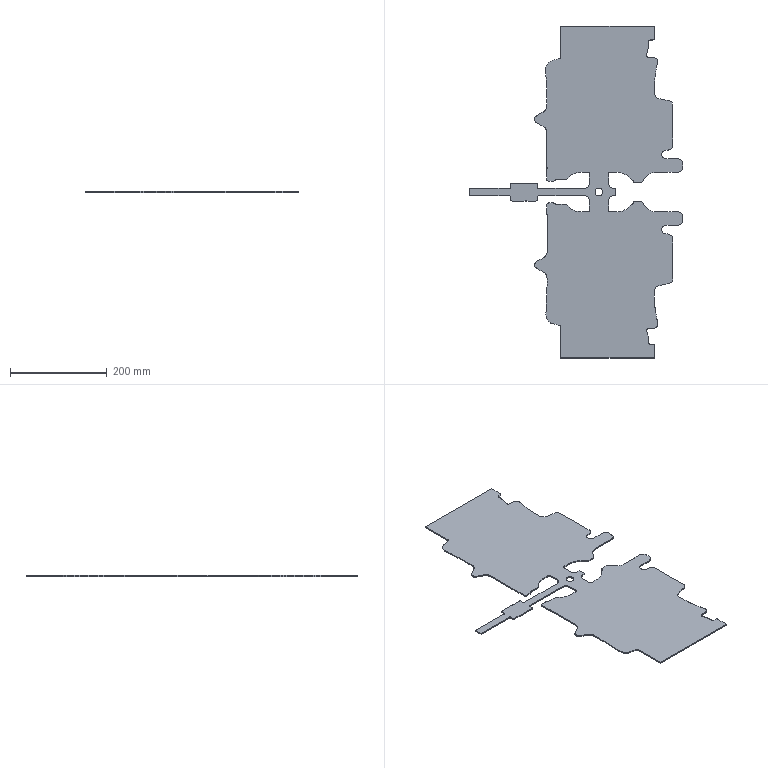Part | STEP file | lll_id50_x_t | 1 solid | 310 faces | box 439.5 x 684.75 x 2.5 mm | volume 383767 mm3 | cylinder 233 | plane 77 | commonest cylinder face diameters 6 x52 20 x14 8 x10 20.001 x4 59.996 x4 17 x2